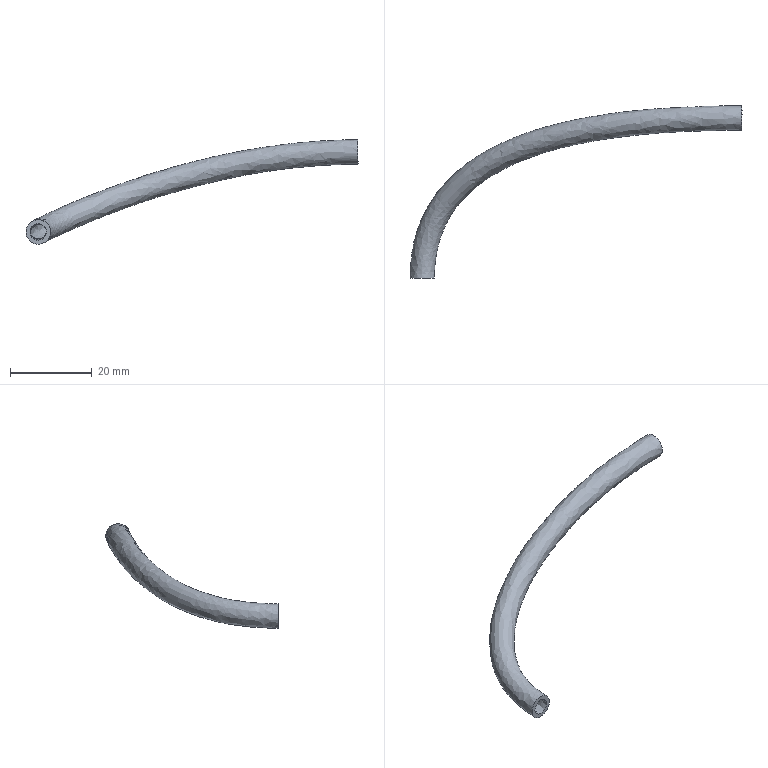Part | NX | features solid 2 | 1 solid | 4 faces | box 81 x 42.023 x 25.5 mm | volume 1564 mm3 | plane 2 | spline 2